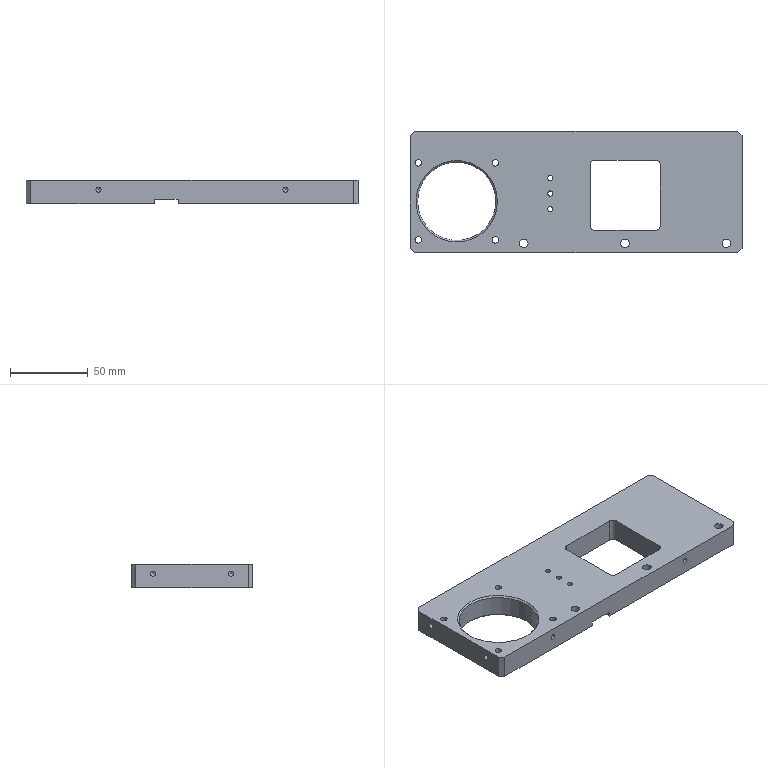Part | 1 solid | 57 faces | box 213 x 78 x 15 mm | volume 181371 mm3 | cylinder 26 | plane 21 | cone 10 | commonest cylinder face diameters 3.3 x11 4.2 x4 6 x4 5.5 x3 10 x3 50.3 x1
STEP:
#1=CARTESIAN_POINT('',(-38.5,-33.,-2.1));
#2=VERTEX_POINT('',#1);
#3=CARTESIAN_POINT('',(-33.5,-33.,-2.1));
#4=DIRECTION('',(0.,0.,-1.));
#5=DIRECTION('',(-1.,0.,0.));
#6=AXIS2_PLACEMENT_3D('',#3,#4,#5);
#7=CIRCLE('',#6,5.);
#8=EDGE_CURVE('',#2,#2,#7,.T.);
#9=ORIENTED_EDGE('',*,*,#8,.T.);
#10=EDGE_LOOP('',(#9));
#11=FACE_BOUND('',#10,.T.);
#12=CARTESIAN_POINT('',(-36.25,-33.,-2.1));
#13=VERTEX_POINT('',#12);
#14=CARTESIAN_POINT('',(-33.5,-33.,-2.1));
#15=DIRECTION('',(0.,0.,-1.));
#16=DIRECTION('',(-1.,0.,0.));
#17=AXIS2_PLACEMENT_3D('',#14,#15,#16);
#18=CIRCLE('',#17,2.75);
#19=EDGE_CURVE('',#13,#13,#18,.T.);
#20=ORIENTED_EDGE('',*,*,#19,.F.);
#21=EDGE_LOOP('',(#20));
#22=FACE_BOUND('',#21,.T.);
#23=CARTESIAN_POINT('',(-30.75,-33.,-2.1));
#24=DIRECTION('',(0.,0.,1.));
#25=DIRECTION('',(1.,0.,0.));
#26=AXIS2_PLACEMENT_3D('',#23,#24,#25);
#27=PLANE('',#26);
#28=ADVANCED_FACE('',(#11,#22),#27,.F.);
#29=CARTESIAN_POINT('',(101.5,-33.,-2.1));
#30=VERTEX_POINT('',#29);
#31=CARTESIAN_POINT('',(96.5,-33.,-2.1));
#32=DIRECTION('',(0.,0.,-1.));
#33=DIRECTION('',(1.,0.,0.));
#34=AXIS2_PLACEMENT_3D('',#31,#32,#33);
#35=CIRCLE('',#34,5.);
#36=EDGE_CURVE('',#30,#30,#35,.T.);
#37=ORIENTED_EDGE('',*,*,#36,.T.);
#38=EDGE_LOOP('',(#37));
#39=FACE_BOUND('',#38,.T.);
#40=CARTESIAN_POINT('',(99.25,-33.,-2.1));
#41=VERTEX_POINT('',#40);
#42=CARTESIAN_POINT('',(96.5,-33.,-2.1));
#43=DIRECTION('',(0.,0.,-1.));
#44=DIRECTION('',(1.,0.,0.));
#45=AXIS2_PLACEMENT_3D('',#42,#43,#44);
#46=CIRCLE('',#45,2.75);
#47=EDGE_CURVE('',#41,#41,#46,.T.);
#48=ORIENTED_EDGE('',*,*,#47,.F.);
#49=EDGE_LOOP('',(#48));
#50=FACE_BOUND('',#49,.T.);
#51=CARTESIAN_POINT('',(-30.75,-33.,-2.1));
#52=DIRECTION('',(0.,0.,1.));
#53=DIRECTION('',(1.,0.,0.));
#54=AXIS2_PLACEMENT_3D('',#51,#52,#53);
#55=PLANE('',#54);
#56=ADVANCED_FACE('',(#39,#50),#55,.F.);
#57=CARTESIAN_POINT('',(36.5,-33.,-2.1));
#58=VERTEX_POINT('',#57);
#59=CARTESIAN_POINT('',(31.5,-33.,-2.1));
#60=DIRECTION('',(0.,0.,-1.));
#61=DIRECTION('',(1.,0.,0.));
#62=AXIS2_PLACEMENT_3D('',#59,#60,#61);
#63=CIRCLE('',#62,5.);
#64=EDGE_CURVE('',#58,#58,#63,.T.);
#65=ORIENTED_EDGE('',*,*,#64,.T.);
#66=EDGE_LOOP('',(#65));
#67=FACE_BOUND('',#66,.T.);
#68=CARTESIAN_POINT('',(34.25,-33.,-2.1));
#69=VERTEX_POINT('',#68);
#70=CARTESIAN_POINT('',(31.5,-33.,-2.1));
#71=DIRECTION('',(0.,0.,-1.));
#72=DIRECTION('',(1.,0.,0.));
#73=AXIS2_PLACEMENT_3D('',#70,#71,#72);
#74=CIRCLE('',#73,2.75);
#75=EDGE_CURVE('',#69,#69,#74,.T.);
#76=ORIENTED_EDGE('',*,*,#75,.F.);
#77=EDGE_LOOP('',(#76));
#78=FACE_BOUND('',#77,.T.);
#79=CARTESIAN_POINT('',(-30.75,-33.,-2.1));
#80=DIRECTION('',(0.,0.,1.));
#81=DIRECTION('',(1.,0.,0.));
#82=AXIS2_PLACEMENT_3D('',#79,#80,#81);
#83=PLANE('',#82);
#84=ADVANCED_FACE('',(#67,#78),#83,.F.);
#85=CARTESIAN_POINT('',(106.5,36.,7.5));
#86=VERTEX_POINT('',#85);
#87=CARTESIAN_POINT('',(103.5,39.,7.5));
#88=VERTEX_POINT('',#87);
#89=CARTESIAN_POINT('',(71.25,71.25,7.5));
#90=DIRECTION('',(-0.7071,0.7071,0.));
#91=VECTOR('',#90,1000.);
#92=LINE('',#89,#91);
#93=EDGE_CURVE('',#86,#88,#92,.T.);
#94=ORIENTED_EDGE('',*,*,#93,.F.);
#95=CARTESIAN_POINT('',(106.5,36.,-7.5));
#96=VERTEX_POINT('',#95);
#97=CARTESIAN_POINT('',(106.5,36.,7.5));
#98=DIRECTION('',(0.,0.,1.));
#99=VECTOR('',#98,1000.);
#100=LINE('',#97,#99);
#101=EDGE_CURVE('',#96,#86,#100,.T.);
#102=ORIENTED_EDGE('',*,*,#101,.F.);
#103=CARTESIAN_POINT('',(103.5,39.,-7.5));
#104=VERTEX_POINT('',#103);
#105=CARTESIAN_POINT('',(103.5,39.,-7.5));
#106=DIRECTION('',(0.7071,-0.7071,0.));
#107=VECTOR('',#106,1000.);
#108=LINE('',#105,#107);
#109=EDGE_CURVE('',#104,#96,#108,.T.);
#110=ORIENTED_EDGE('',*,*,#109,.F.);
#111=CARTESIAN_POINT('',(103.5,39.,7.5));
#112=DIRECTION('',(0.,0.,-1.));
#113=VECTOR('',#112,1000.);
#114=LINE('',#111,#113);
#115=EDGE_CURVE('',#88,#104,#114,.T.);
#116=ORIENTED_EDGE('',*,*,#115,.F.);
#117=EDGE_LOOP('',(#94,#102,#110,#116));
#118=FACE_BOUND('',#117,.T.);
#119=CARTESIAN_POINT('',(103.5,39.,7.5));
#120=DIRECTION('',(-0.7071,-0.7071,0.));
#121=DIRECTION('',(0.,0.,-1.));
#122=AXIS2_PLACEMENT_3D('',#119,#120,#121);
#123=PLANE('',#122);
#124=ADVANCED_FACE('',(#118),#123,.F.);
#125=CARTESIAN_POINT('',(103.5,-39.,7.5));
#126=VERTEX_POINT('',#125);
#127=CARTESIAN_POINT('',(106.5,-36.,7.5));
#128=VERTEX_POINT('',#127);
#129=CARTESIAN_POINT('',(71.25,-71.25,7.5));
#130=DIRECTION('',(0.7071,0.7071,0.));
#131=VECTOR('',#130,1000.);
#132=LINE('',#129,#131);
#133=EDGE_CURVE('',#126,#128,#132,.T.);
#134=ORIENTED_EDGE('',*,*,#133,.F.);
#135=CARTESIAN_POINT('',(103.5,-39.,-7.5));
#136=VERTEX_POINT('',#135);
#137=CARTESIAN_POINT('',(103.5,-39.,7.5));
#138=DIRECTION('',(0.,0.,1.));
#139=VECTOR('',#138,1000.);
#140=LINE('',#137,#139);
#141=EDGE_CURVE('',#136,#126,#140,.T.);
#142=ORIENTED_EDGE('',*,*,#141,.F.);
#143=CARTESIAN_POINT('',(106.5,-36.,-7.5));
#144=VERTEX_POINT('',#143);
#145=CARTESIAN_POINT('',(106.5,-36.,-7.5));
#146=DIRECTION('',(-0.7071,-0.7071,0.));
#147=VECTOR('',#146,1000.);
#148=LINE('',#145,#147);
#149=EDGE_CURVE('',#144,#136,#148,.T.);
#150=ORIENTED_EDGE('',*,*,#149,.F.);
#151=CARTESIAN_POINT('',(106.5,-36.,7.5));
#152=DIRECTION('',(0.,0.,-1.));
#153=VECTOR('',#152,1000.);
#154=LINE('',#151,#153);
#155=EDGE_CURVE('',#128,#144,#154,.T.);
#156=ORIENTED_EDGE('',*,*,#155,.F.);
#157=EDGE_LOOP('',(#134,#142,#150,#156));
#158=FACE_BOUND('',#157,.T.);
#159=CARTESIAN_POINT('',(106.5,-36.,7.5));
#160=DIRECTION('',(-0.7071,0.7071,0.));
#161=DIRECTION('',(0.,0.,-1.));
#162=AXIS2_PLACEMENT_3D('',#159,#160,#161);
#163=PLANE('',#162);
#164=ADVANCED_FACE('',(#158),#163,.F.);
#165=CARTESIAN_POINT('',(-103.5,39.,7.5));
#166=VERTEX_POINT('',#165);
#167=CARTESIAN_POINT('',(-106.5,36.,7.5));
#168=VERTEX_POINT('',#167);
#169=CARTESIAN_POINT('',(-71.25,71.25,7.5));
#170=DIRECTION('',(-0.7071,-0.7071,0.));
#171=VECTOR('',#170,1000.);
#172=LINE('',#169,#171);
#173=EDGE_CURVE('',#166,#168,#172,.T.);
#174=ORIENTED_EDGE('',*,*,#173,.F.);
#175=CARTESIAN_POINT('',(-103.5,39.,-7.5));
#176=VERTEX_POINT('',#175);
#177=CARTESIAN_POINT('',(-103.5,39.,7.5));
#178=DIRECTION('',(0.,0.,1.));
#179=VECTOR('',#178,1000.);
#180=LINE('',#177,#179);
#181=EDGE_CURVE('',#176,#166,#180,.T.);
#182=ORIENTED_EDGE('',*,*,#181,.F.);
#183=CARTESIAN_POINT('',(-106.5,36.,-7.5));
#184=VERTEX_POINT('',#183);
#185=CARTESIAN_POINT('',(-106.5,36.,-7.5));
#186=DIRECTION('',(0.7071,0.7071,0.));
#187=VECTOR('',#186,1000.);
#188=LINE('',#185,#187);
#189=EDGE_CURVE('',#184,#176,#188,.T.);
#190=ORIENTED_EDGE('',*,*,#189,.F.);
#191=CARTESIAN_POINT('',(-106.5,36.,7.5));
#192=DIRECTION('',(0.,0.,-1.));
#193=VECTOR('',#192,1000.);
#194=LINE('',#191,#193);
#195=EDGE_CURVE('',#168,#184,#194,.T.);
#196=ORIENTED_EDGE('',*,*,#195,.F.);
#197=EDGE_LOOP('',(#174,#182,#190,#196));
#198=FACE_BOUND('',#197,.T.);
#199=CARTESIAN_POINT('',(-106.5,36.,7.5));
#200=DIRECTION('',(0.7071,-0.7071,0.));
#201=DIRECTION('',(0.,0.,-1.));
#202=AXIS2_PLACEMENT_3D('',#199,#200,#201);
#203=PLANE('',#202);
#204=ADVANCED_FACE('',(#198),#203,.F.);
#205=CARTESIAN_POINT('',(-106.5,-36.,7.5));
#206=VERTEX_POINT('',#205);
#207=CARTESIAN_POINT('',(-103.5,-39.,7.5));
#208=VERTEX_POINT('',#207);
#209=CARTESIAN_POINT('',(-71.25,-71.25,7.5));
#210=DIRECTION('',(0.7071,-0.7071,0.));
#211=VECTOR('',#210,1000.);
#212=LINE('',#209,#211);
#213=EDGE_CURVE('',#206,#208,#212,.T.);
#214=ORIENTED_EDGE('',*,*,#213,.F.);
#215=CARTESIAN_POINT('',(-106.5,-36.,-7.5));
#216=VERTEX_POINT('',#215);
#217=CARTESIAN_POINT('',(-106.5,-36.,7.5));
#218=DIRECTION('',(0.,0.,1.));
#219=VECTOR('',#218,1000.);
#220=LINE('',#217,#219);
#221=EDGE_CURVE('',#216,#206,#220,.T.);
#222=ORIENTED_EDGE('',*,*,#221,.F.);
#223=CARTESIAN_POINT('',(-103.5,-39.,-7.5));
#224=VERTEX_POINT('',#223);
#225=CARTESIAN_POINT('',(-103.5,-39.,-7.5));
#226=DIRECTION('',(-0.7071,0.7071,0.));
#227=VECTOR('',#226,1000.);
#228=LINE('',#225,#227);
#229=EDGE_CURVE('',#224,#216,#228,.T.);
#230=ORIENTED_EDGE('',*,*,#229,.F.);
#231=CARTESIAN_POINT('',(-103.5,-39.,7.5));
#232=DIRECTION('',(0.,0.,-1.));
#233=VECTOR('',#232,1000.);
#234=LINE('',#231,#233);
#235=EDGE_CURVE('',#208,#224,#234,.T.);
#236=ORIENTED_EDGE('',*,*,#235,.F.);
#237=EDGE_LOOP('',(#214,#222,#230,#236));
#238=FACE_BOUND('',#237,.T.);
#239=CARTESIAN_POINT('',(-103.5,-39.,7.5));
#240=DIRECTION('',(0.7071,0.7071,0.));
#241=DIRECTION('',(0.,0.,-1.));
#242=AXIS2_PLACEMENT_3D('',#239,#240,#241);
#243=PLANE('',#242);
#244=ADVANCED_FACE('',(#238),#243,.F.);
#245=CARTESIAN_POINT('',(51.,20.5,7.5));
#246=VERTEX_POINT('',#245);
#247=CARTESIAN_POINT('',(54.,17.5,7.5));
#248=VERTEX_POINT('',#247);
#249=CARTESIAN_POINT('',(51.,17.5,7.5));
#250=DIRECTION('',(0.,0.,-1.));
#251=DIRECTION('',(1.,0.,0.));
#252=AXIS2_PLACEMENT_3D('',#249,#250,#251);
#253=CIRCLE('',#252,3.);
#254=EDGE_CURVE('',#246,#248,#253,.T.);
#255=ORIENTED_EDGE('',*,*,#254,.F.);
#256=CARTESIAN_POINT('',(51.,20.5,-7.5));
#257=VERTEX_POINT('',#256);
#258=CARTESIAN_POINT('',(51.,20.5,7.5));
#259=DIRECTION('',(0.,0.,1.));
#260=VECTOR('',#259,1000.);
#261=LINE('',#258,#260);
#262=EDGE_CURVE('',#257,#246,#261,.T.);
#263=ORIENTED_EDGE('',*,*,#262,.F.);
#264=CARTESIAN_POINT('',(54.,17.5,-7.5));
#265=VERTEX_POINT('',#264);
#266=CARTESIAN_POINT('',(51.,17.5,-7.5));
#267=DIRECTION('',(0.,0.,1.));
#268=DIRECTION('',(1.,0.,0.));
#269=AXIS2_PLACEMENT_3D('',#266,#267,#268);
#270=CIRCLE('',#269,3.);
#271=EDGE_CURVE('',#265,#257,#270,.T.);
#272=ORIENTED_EDGE('',*,*,#271,.F.);
#273=CARTESIAN_POINT('',(54.,17.5,-7.5));
#274=DIRECTION('',(0.,0.,-1.));
#275=VECTOR('',#274,1000.);
#276=LINE('',#273,#275);
#277=EDGE_CURVE('',#248,#265,#276,.T.);
#278=ORIENTED_EDGE('',*,*,#277,.F.);
#279=EDGE_LOOP('',(#255,#263,#272,#278));
#280=FACE_BOUND('',#279,.T.);
#281=CARTESIAN_POINT('',(51.,17.5,7.5));
#282=DIRECTION('',(0.,0.,1.));
#283=DIRECTION('',(1.,0.,0.));
#284=AXIS2_PLACEMENT_3D('',#281,#282,#283);
#285=CYLINDRICAL_SURFACE('',#284,3.);
#286=ADVANCED_FACE('',(#280),#285,.F.);
#287=CARTESIAN_POINT('',(54.,-21.5,7.5));
#288=VERTEX_POINT('',#287);
#289=CARTESIAN_POINT('',(51.,-24.5,7.5));
#290=VERTEX_POINT('',#289);
#291=CARTESIAN_POINT('',(51.,-21.5,7.5));
#292=DIRECTION('',(0.,0.,-1.));
#293=DIRECTION('',(1.,0.,0.));
#294=AXIS2_PLACEMENT_3D('',#291,#292,#293);
#295=CIRCLE('',#294,3.);
#296=EDGE_CURVE('',#288,#290,#295,.T.);
#297=ORIENTED_EDGE('',*,*,#296,.F.);
#298=CARTESIAN_POINT('',(54.,-21.5,-7.5));
#299=VERTEX_POINT('',#298);
#300=CARTESIAN_POINT('',(54.,-21.5,7.5));
#301=DIRECTION('',(0.,0.,1.));
#302=VECTOR('',#301,1000.);
#303=LINE('',#300,#302);
#304=EDGE_CURVE('',#299,#288,#303,.T.);
#305=ORIENTED_EDGE('',*,*,#304,.F.);
#306=CARTESIAN_POINT('',(51.,-24.5,-7.5));
#307=VERTEX_POINT('',#306);
#308=CARTESIAN_POINT('',(51.,-21.5,-7.5));
#309=DIRECTION('',(0.,0.,1.));
#310=DIRECTION('',(1.,0.,0.));
#311=AXIS2_PLACEMENT_3D('',#308,#309,#310);
#312=CIRCLE('',#311,3.);
#313=EDGE_CURVE('',#307,#299,#312,.T.);
#314=ORIENTED_EDGE('',*,*,#313,.F.);
#315=CARTESIAN_POINT('',(51.,-24.5,-7.5));
#316=DIRECTION('',(0.,0.,-1.));
#317=VECTOR('',#316,1000.);
#318=LINE('',#315,#317);
#319=EDGE_CURVE('',#290,#307,#318,.T.);
#320=ORIENTED_EDGE('',*,*,#319,.F.);
#321=EDGE_LOOP('',(#297,#305,#314,#320));
#322=FACE_BOUND('',#321,.T.);
#323=CARTESIAN_POINT('',(51.,-21.5,7.5));
#324=DIRECTION('',(0.,0.,1.));
#325=DIRECTION('',(1.,0.,0.));
#326=AXIS2_PLACEMENT_3D('',#323,#324,#325);
#327=CYLINDRICAL_SURFACE('',#326,3.);
#328=ADVANCED_FACE('',(#322),#327,.F.);
#329=CARTESIAN_POINT('',(12.,-24.5,7.5));
#330=VERTEX_POINT('',#329);
#331=CARTESIAN_POINT('',(9.,-21.5,7.5));
#332=VERTEX_POINT('',#331);
#333=CARTESIAN_POINT('',(12.,-21.5,7.5));
#334=DIRECTION('',(0.,0.,-1.));
#335=DIRECTION('',(1.,0.,0.));
#336=AXIS2_PLACEMENT_3D('',#333,#334,#335);
#337=CIRCLE('',#336,3.);
#338=EDGE_CURVE('',#330,#332,#337,.T.);
#339=ORIENTED_EDGE('',*,*,#338,.F.);
#340=CARTESIAN_POINT('',(12.,-24.5,-7.5));
#341=VERTEX_POINT('',#340);
#342=CARTESIAN_POINT('',(12.,-24.5,7.5));
#343=DIRECTION('',(0.,0.,1.));
#344=VECTOR('',#343,1000.);
#345=LINE('',#342,#344);
#346=EDGE_CURVE('',#341,#330,#345,.T.);
#347=ORIENTED_EDGE('',*,*,#346,.F.);
#348=CARTESIAN_POINT('',(9.,-21.5,-7.5));
#349=VERTEX_POINT('',#348);
#350=CARTESIAN_POINT('',(12.,-21.5,-7.5));
#351=DIRECTION('',(0.,0.,1.));
#352=DIRECTION('',(1.,0.,0.));
#353=AXIS2_PLACEMENT_3D('',#350,#351,#352);
#354=CIRCLE('',#353,3.);
#355=EDGE_CURVE('',#349,#341,#354,.T.);
#356=ORIENTED_EDGE('',*,*,#355,.F.);
#357=CARTESIAN_POINT('',(9.,-21.5,-7.5));
#358=DIRECTION('',(0.,0.,-1.));
#359=VECTOR('',#358,1000.);
#360=LINE('',#357,#359);
#361=EDGE_CURVE('',#332,#349,#360,.T.);
#362=ORIENTED_EDGE('',*,*,#361,.F.);
#363=EDGE_LOOP('',(#339,#347,#356,#362));
#364=FACE_BOUND('',#363,.T.);
#365=CARTESIAN_POINT('',(12.,-21.5,7.5));
#366=DIRECTION('',(0.,0.,1.));
#367=DIRECTION('',(1.,0.,0.));
#368=AXIS2_PLACEMENT_3D('',#365,#366,#367);
#369=CYLINDRICAL_SURFACE('',#368,3.);
#370=ADVANCED_FACE('',(#364),#369,.F.);
#371=CARTESIAN_POINT('',(9.,17.5,7.5));
#372=VERTEX_POINT('',#371);
#373=CARTESIAN_POINT('',(12.,20.5,7.5));
#374=VERTEX_POINT('',#373);
#375=CARTESIAN_POINT('',(12.,17.5,7.5));
#376=DIRECTION('',(0.,0.,-1.));
#377=DIRECTION('',(1.,0.,0.));
#378=AXIS2_PLACEMENT_3D('',#375,#376,#377);
#379=CIRCLE('',#378,3.);
#380=EDGE_CURVE('',#372,#374,#379,.T.);
#381=ORIENTED_EDGE('',*,*,#380,.F.);
#382=CARTESIAN_POINT('',(9.,17.5,-7.5));
#383=VERTEX_POINT('',#382);
#384=CARTESIAN_POINT('',(9.,17.5,7.5));
#385=DIRECTION('',(0.,0.,1.));
#386=VECTOR('',#385,1000.);
#387=LINE('',#384,#386);
#388=EDGE_CURVE('',#383,#372,#387,.T.);
#389=ORIENTED_EDGE('',*,*,#388,.F.);
#390=CARTESIAN_POINT('',(12.,20.5,-7.5));
#391=VERTEX_POINT('',#390);
#392=CARTESIAN_POINT('',(12.,17.5,-7.5));
#393=DIRECTION('',(0.,0.,1.));
#394=DIRECTION('',(1.,0.,0.));
#395=AXIS2_PLACEMENT_3D('',#392,#393,#394);
#396=CIRCLE('',#395,3.);
#397=EDGE_CURVE('',#391,#383,#396,.T.);
#398=ORIENTED_EDGE('',*,*,#397,.F.);
#399=CARTESIAN_POINT('',(12.,20.5,-7.5));
#400=DIRECTION('',(0.,0.,-1.));
#401=VECTOR('',#400,1000.);
#402=LINE('',#399,#401);
#403=EDGE_CURVE('',#374,#391,#402,.T.);
#404=ORIENTED_EDGE('',*,*,#403,.F.);
#405=EDGE_LOOP('',(#381,#389,#398,#404));
#406=FACE_BOUND('',#405,.T.);
#407=CARTESIAN_POINT('',(12.,17.5,7.5));
#408=DIRECTION('',(0.,0.,1.));
#409=DIRECTION('',(1.,0.,0.));
#410=AXIS2_PLACEMENT_3D('',#407,#408,#409);
#411=CYLINDRICAL_SURFACE('',#410,3.);
#412=ADVANCED_FACE('',(#406),#411,.F.);
#413=CARTESIAN_POINT('',(54.,20.5,7.5));
#414=DIRECTION('',(1.,0.,0.));
#415=VECTOR('',#414,1000.);
#416=LINE('',#413,#415);
#417=EDGE_CURVE('',#374,#246,#416,.T.);
#418=ORIENTED_EDGE('',*,*,#417,.F.);
#419=ORIENTED_EDGE('',*,*,#403,.T.);
#420=CARTESIAN_POINT('',(54.,20.5,-7.5));
#421=DIRECTION('',(1.,0.,0.));
#422=VECTOR('',#421,1000.);
#423=LINE('',#420,#422);
#424=EDGE_CURVE('',#391,#257,#423,.T.);
#425=ORIENTED_EDGE('',*,*,#424,.T.);
#426=ORIENTED_EDGE('',*,*,#262,.T.);
#427=EDGE_LOOP('',(#418,#419,#425,#426));
#428=FACE_BOUND('',#427,.T.);
#429=CARTESIAN_POINT('',(54.,20.5,7.5));
#430=DIRECTION('',(0.,1.,0.));
#431=DIRECTION('',(0.,0.,1.));
#432=AXIS2_PLACEMENT_3D('',#429,#430,#431);
#433=PLANE('',#432);
#434=ADVANCED_FACE('',(#428),#433,.F.);
#435=CARTESIAN_POINT('',(54.,20.5,-7.5));
#436=DIRECTION('',(0.,-1.,0.));
#437=VECTOR('',#436,1000.);
#438=LINE('',#435,#437);
#439=EDGE_CURVE('',#265,#299,#438,.T.);
#440=ORIENTED_EDGE('',*,*,#439,.T.);
#441=ORIENTED_EDGE('',*,*,#304,.T.);
#442=CARTESIAN_POINT('',(54.,20.5,7.5));
#443=DIRECTION('',(0.,-1.,0.));
#444=VECTOR('',#443,1000.);
#445=LINE('',#442,#444);
#446=EDGE_CURVE('',#248,#288,#445,.T.);
#447=ORIENTED_EDGE('',*,*,#446,.F.);
#448=ORIENTED_EDGE('',*,*,#277,.T.);
#449=EDGE_LOOP('',(#440,#441,#447,#448));
#450=FACE_BOUND('',#449,.T.);
#451=CARTESIAN_POINT('',(54.,20.5,7.5));
#452=DIRECTION('',(1.,0.,0.));
#453=DIRECTION('',(0.,1.,0.));
#454=AXIS2_PLACEMENT_3D('',#451,#452,#453);
#455=PLANE('',#454);
#456=ADVANCED_FACE('',(#450),#455,.F.);
#457=CARTESIAN_POINT('',(54.,-24.5,-7.5));
#458=DIRECTION('',(-1.,0.,0.));
#459=VECTOR('',#458,1000.);
#460=LINE('',#457,#459);
#461=EDGE_CURVE('',#307,#341,#460,.T.);
#462=ORIENTED_EDGE('',*,*,#461,.T.);
#463=ORIENTED_EDGE('',*,*,#346,.T.);
#464=CARTESIAN_POINT('',(54.,-24.5,7.5));
#465=DIRECTION('',(-1.,0.,0.));
#466=VECTOR('',#465,1000.);
#467=LINE('',#464,#466);
#468=EDGE_CURVE('',#290,#330,#467,.T.);
#469=ORIENTED_EDGE('',*,*,#468,.F.);
#470=ORIENTED_EDGE('',*,*,#319,.T.);
#471=EDGE_LOOP('',(#462,#463,#469,#470));
#472=FACE_BOUND('',#471,.T.);
#473=CARTESIAN_POINT('',(54.,-24.5,7.5));
#474=DIRECTION('',(0.,-1.,0.));
#475=DIRECTION('',(0.,0.,-1.));
#476=AXIS2_PLACEMENT_3D('',#473,#474,#475);
#477=PLANE('',#476);
#478=ADVANCED_FACE('',(#472),#477,.F.);
#479=CARTESIAN_POINT('',(9.,20.5,-7.5));
#480=DIRECTION('',(0.,1.,0.));
#481=VECTOR('',#480,1000.);
#482=LINE('',#479,#481);
#483=EDGE_CURVE('',#349,#383,#482,.T.);
#484=ORIENTED_EDGE('',*,*,#483,.T.);
#485=ORIENTED_EDGE('',*,*,#388,.T.);
#486=CARTESIAN_POINT('',(9.,20.5,7.5));
#487=DIRECTION('',(0.,1.,0.));
#488=VECTOR('',#487,1000.);
#489=LINE('',#486,#488);
#490=EDGE_CURVE('',#332,#372,#489,.T.);
#491=ORIENTED_EDGE('',*,*,#490,.F.);
#492=ORIENTED_EDGE('',*,*,#361,.T.);
#493=EDGE_LOOP('',(#484,#485,#491,#492));
#494=FACE_BOUND('',#493,.T.);
#495=CARTESIAN_POINT('',(9.,20.5,7.5));
#496=DIRECTION('',(-1.,0.,0.));
#497=DIRECTION('',(0.,-1.,0.));
#498=AXIS2_PLACEMENT_3D('',#495,#496,#497);
#499=PLANE('',#498);
#500=ADVANCED_FACE('',(#494),#499,.F.);
#501=CARTESIAN_POINT('',(-8.95,39.,-4.5));
#502=VERTEX_POINT('',#501);
#503=CARTESIAN_POINT('',(-8.95,-39.,-4.5));
#504=VERTEX_POINT('',#503);
#505=CARTESIAN_POINT('',(-8.95,39.,-4.5));
#506=DIRECTION('',(0.,-1.,0.));
#507=VECTOR('',#506,1000.);
#508=LINE('',#505,#507);
#509=EDGE_CURVE('',#502,#504,#508,.T.);
#510=ORIENTED_EDGE('',*,*,#509,.T.);
#511=CARTESIAN_POINT('',(-24.05,-39.,-4.5));
#512=VERTEX_POINT('',#511);
#513=CARTESIAN_POINT('',(-8.95,-39.,-4.5));
#514=DIRECTION('',(-1.,0.,0.));
#515=VECTOR('',#514,1000.);
#516=LINE('',#513,#515);
#517=EDGE_CURVE('',#504,#512,#516,.T.);
#518=ORIENTED_EDGE('',*,*,#517,.T.);
#519=CARTESIAN_POINT('',(-24.05,39.,-4.5));
#520=VERTEX_POINT('',#519);
#521=CARTESIAN_POINT('',(-24.05,39.,-4.5));
#522=DIRECTION('',(0.,1.,0.));
#523=VECTOR('',#522,1000.);
#524=LINE('',#521,#523);
#525=EDGE_CURVE('',#512,#520,#524,.T.);
#526=ORIENTED_EDGE('',*,*,#525,.T.);
#527=CARTESIAN_POINT('',(-8.95,39.,-4.5));
#528=DIRECTION('',(1.,0.,0.));
#529=VECTOR('',#528,1000.);
#530=LINE('',#527,#529);
#531=EDGE_CURVE('',#520,#502,#530,.T.);
#532=ORIENTED_EDGE('',*,*,#531,.T.);
#533=EDGE_LOOP('',(#510,#518,#526,#532));
#534=FACE_BOUND('',#533,.T.);
#535=CARTESIAN_POINT('',(-18.15,-11.,-4.5));
#536=VERTEX_POINT('',#535);
#537=CARTESIAN_POINT('',(-16.5,-11.,-4.5));
#538=DIRECTION('',(0.,0.,-1.));
#539=DIRECTION('',(-1.,0.,0.));
#540=AXIS2_PLACEMENT_3D('',#537,#538,#539);
#541=CIRCLE('',#540,1.65);
#542=EDGE_CURVE('',#536,#536,#541,.T.);
#543=ORIENTED_EDGE('',*,*,#542,.F.);
#544=EDGE_LOOP('',(#543));
#545=FACE_BOUND('',#544,.T.);
#546=CARTESIAN_POINT('',(-18.15,9.,-4.5));
#547=VERTEX_POINT('',#546);
#548=CARTESIAN_POINT('',(-16.5,9.,-4.5));
#549=DIRECTION('',(0.,0.,-1.));
#550=DIRECTION('',(-1.,0.,0.));
#551=AXIS2_PLACEMENT_3D('',#548,#549,#550);
#552=CIRCLE('',#551,1.65);
#553=EDGE_CURVE('',#547,#547,#552,.T.);
#554=ORIENTED_EDGE('',*,*,#553,.F.);
#555=EDGE_LOOP('',(#554));
#556=FACE_BOUND('',#555,.T.);
#557=CARTESIAN_POINT('',(-18.15,-1.,-4.5));
#558=VERTEX_POINT('',#557);
#559=CARTESIAN_POINT('',(-16.5,-1.,-4.5));
#560=DIRECTION('',(0.,0.,-1.));
#561=DIRECTION('',(-1.,0.,0.));
#562=AXIS2_PLACEMENT_3D('',#559,#560,#561);
#563=CIRCLE('',#562,1.65);
#564=EDGE_CURVE('',#558,#558,#563,.T.);
#565=ORIENTED_EDGE('',*,*,#564,.F.);
#566=EDGE_LOOP('',(#565));
#567=FACE_BOUND('',#566,.T.);
#568=CARTESIAN_POINT('',(0.,0.,-4.5));
#569=DIRECTION('',(0.,0.,-1.));
#570=DIRECTION('',(-1.,0.,0.));
#571=AXIS2_PLACEMENT_3D('',#568,#569,#570);
#572=PLANE('',#571);
#573=ADVANCED_FACE('',(#534,#545,#556,#567),#572,.T.);
#574=CARTESIAN_POINT('',(-24.05,-39.,-7.5));
#575=VERTEX_POINT('',#574);
#576=CARTESIAN_POINT('',(-24.05,39.,-7.5));
#577=VERTEX_POINT('',#576);
#578=CARTESIAN_POINT('',(-24.05,39.,-7.5));
#579=DIRECTION('',(0.,1.,0.));
#580=VECTOR('',#579,1000.);
#581=LINE('',#578,#580);
#582=EDGE_CURVE('',#575,#577,#581,.T.);
#583=ORIENTED_EDGE('',*,*,#582,.T.);
#584=CARTESIAN_POINT('',(-24.05,39.,-4.5));
#585=DIRECTION('',(0.,0.,-1.));
#586=VECTOR('',#585,1000.);
#587=LINE('',#584,#586);
#588=EDGE_CURVE('',#520,#577,#587,.T.);
#589=ORIENTED_EDGE('',*,*,#588,.F.);
#590=ORIENTED_EDGE('',*,*,#525,.F.);
#591=CARTESIAN_POINT('',(-24.05,-39.,-4.5));
#592=DIRECTION('',(0.,0.,-1.));
#593=VECTOR('',#592,1000.);
#594=LINE('',#591,#593);
#595=EDGE_CURVE('',#512,#575,#594,.T.);
#596=ORIENTED_EDGE('',*,*,#595,.T.);
#597=EDGE_LOOP('',(#583,#589,#590,#596));
#598=FACE_BOUND('',#597,.T.);
#599=CARTESIAN_POINT('',(-24.05,39.,-4.5));
#600=DIRECTION('',(-1.,0.,0.));
#601=DIRECTION('',(0.,-1.,0.));
#602=AXIS2_PLACEMENT_3D('',#599,#600,#601);
#603=PLANE('',#602);
#604=ADVANCED_FACE('',(#598),#603,.F.);
#605=CARTESIAN_POINT('',(-8.95,39.,-7.5));
#606=VERTEX_POINT('',#605);
#607=CARTESIAN_POINT('',(-8.95,-39.,-7.5));
#608=VERTEX_POINT('',#607);
#609=CARTESIAN_POINT('',(-8.95,39.,-7.5));
#610=DIRECTION('',(0.,-1.,0.));
#611=VECTOR('',#610,1000.);
#612=LINE('',#609,#611);
#613=EDGE_CURVE('',#606,#608,#612,.T.);
#614=ORIENTED_EDGE('',*,*,#613,.T.);
#615=CARTESIAN_POINT('',(-8.95,-39.,-4.5));
#616=DIRECTION('',(0.,0.,-1.));
#617=VECTOR('',#616,1000.);
#618=LINE('',#615,#617);
#619=EDGE_CURVE('',#504,#608,#618,.T.);
#620=ORIENTED_EDGE('',*,*,#619,.F.);
#621=ORIENTED_EDGE('',*,*,#509,.F.);
#622=CARTESIAN_POINT('',(-8.95,39.,-4.5));
#623=DIRECTION('',(0.,0.,-1.));
#624=VECTOR('',#623,1000.);
#625=LINE('',#622,#624);
#626=EDGE_CURVE('',#502,#606,#625,.T.);
#627=ORIENTED_EDGE('',*,*,#626,.T.);
#628=EDGE_LOOP('',(#614,#620,#621,#627));
#629=FACE_BOUND('',#628,.T.);
#630=CARTESIAN_POINT('',(-8.95,39.,-4.5));
#631=DIRECTION('',(1.,0.,0.));
#632=DIRECTION('',(0.,1.,0.));
#633=AXIS2_PLACEMENT_3D('',#630,#631,#632);
#634=PLANE('',#633);
#635=ADVANCED_FACE('',(#629),#634,.F.);
#636=CARTESIAN_POINT('',(-106.5,-39.,-7.5));
#637=DIRECTION('',(1.,0.,0.));
#638=VECTOR('',#637,1000.);
#639=LINE('',#636,#638);
#640=EDGE_CURVE('',#224,#575,#639,.T.);
#641=ORIENTED_EDGE('',*,*,#640,.F.);
#642=ORIENTED_EDGE('',*,*,#229,.T.);
#643=CARTESIAN_POINT('',(-106.5,39.,-7.5));
#644=DIRECTION('',(0.,-1.,0.));
#645=VECTOR('',#644,1000.);
#646=LINE('',#643,#645);
#647=EDGE_CURVE('',#184,#216,#646,.T.);
#648=ORIENTED_EDGE('',*,*,#647,.F.);
#649=ORIENTED_EDGE('',*,*,#189,.T.);
#650=CARTESIAN_POINT('',(-106.5,39.,-7.5));
#651=DIRECTION('',(-1.,0.,0.));
#652=VECTOR('',#651,1000.);
#653=LINE('',#650,#652);
#654=EDGE_CURVE('',#577,#176,#653,.T.);
#655=ORIENTED_EDGE('',*,*,#654,.F.);
#656=ORIENTED_EDGE('',*,*,#582,.F.);
#657=EDGE_LOOP('',(#641,#642,#648,#649,#655,#656));
#658=FACE_BOUND('',#657,.T.);
#659=CARTESIAN_POINT('',(-99.149,-30.749,-7.5));
#660=VERTEX_POINT('',#659);
#661=CARTESIAN_POINT('',(-101.249,-30.749,-7.5));
#662=DIRECTION('',(0.,0.,1.));
#663=DIRECTION('',(1.,0.,0.));
#664=AXIS2_PLACEMENT_3D('',#661,#662,#663);
#665=CIRCLE('',#664,2.1);
#666=EDGE_CURVE('',#660,#660,#665,.T.);
#667=ORIENTED_EDGE('',*,*,#666,.T.);
#668=EDGE_LOOP('',(#667));
#669=FACE_BOUND('',#668,.T.);
#670=CARTESIAN_POINT('',(-49.651,-30.749,-7.5));
#671=VERTEX_POINT('',#670);
#672=CARTESIAN_POINT('',(-51.751,-30.749,-7.5));
#673=DIRECTION('',(0.,0.,1.));
#674=DIRECTION('',(1.,0.,0.));
#675=AXIS2_PLACEMENT_3D('',#672,#673,#674);
#676=CIRCLE('',#675,2.1);
#677=EDGE_CURVE('',#671,#671,#676,.T.);
#678=ORIENTED_EDGE('',*,*,#677,.T.);
#679=EDGE_LOOP('',(#678));
#680=FACE_BOUND('',#679,.T.);
#681=CARTESIAN_POINT('',(-49.651,18.749,-7.5));
#682=VERTEX_POINT('',#681);
#683=CARTESIAN_POINT('',(-51.751,18.749,-7.5));
#684=DIRECTION('',(0.,0.,1.));
#685=DIRECTION('',(1.,0.,0.));
#686=AXIS2_PLACEMENT_3D('',#683,#684,#685);
#687=CIRCLE('',#686,2.1);
#688=EDGE_CURVE('',#682,#682,#687,.T.);
#689=ORIENTED_EDGE('',*,*,#688,.T.);
#690=EDGE_LOOP('',(#689));
#691=FACE_BOUND('',#690,.T.);
#692=CARTESIAN_POINT('',(-99.149,18.749,-7.5));
#693=VERTEX_POINT('',#692);
#694=CARTESIAN_POINT('',(-101.249,18.749,-7.5));
#695=DIRECTION('',(0.,0.,1.));
#696=DIRECTION('',(1.,0.,0.));
#697=AXIS2_PLACEMENT_3D('',#694,#695,#696);
#698=CIRCLE('',#697,2.1);
#699=EDGE_CURVE('',#693,#693,#698,.T.);
#700=ORIENTED_EDGE('',*,*,#699,.T.);
#701=EDGE_LOOP('',(#700));
#702=FACE_BOUND('',#701,.T.);
#703=CARTESIAN_POINT('',(-38.5,-33.,-7.5));
#704=VERTEX_POINT('',#703);
#705=CARTESIAN_POINT('',(-33.5,-33.,-7.5));
#706=DIRECTION('',(0.,0.,-1.));
#707=DIRECTION('',(-1.,0.,0.));
#708=AXIS2_PLACEMENT_3D('',#705,#706,#707);
#709=CIRCLE('',#708,5.);
#710=EDGE_CURVE('',#704,#704,#709,.T.);
#711=ORIENTED_EDGE('',*,*,#710,.F.);
#712=EDGE_LOOP('',(#711));
#713=FACE_BOUND('',#712,.T.);
#714=CARTESIAN_POINT('',(-50.35,-6.,-7.5));
#715=VERTEX_POINT('',#714);
#716=CARTESIAN_POINT('',(-76.5,-6.,-7.5));
#717=DIRECTION('',(0.,0.,1.));
#718=DIRECTION('',(1.,0.,0.));
#719=AXIS2_PLACEMENT_3D('',#716,#717,#718);
#720=CIRCLE('',#719,26.15);
#721=EDGE_CURVE('',#715,#715,#720,.T.);
#722=ORIENTED_EDGE('',*,*,#721,.T.);
#723=EDGE_LOOP('',(#722));
#724=FACE_BOUND('',#723,.T.);
#725=CARTESIAN_POINT('',(0.,0.,-7.5));
#726=DIRECTION('',(0.,0.,1.));
#727=DIRECTION('',(1.,0.,0.));
#728=AXIS2_PLACEMENT_3D('',#725,#726,#727);
#729=PLANE('',#728);
#730=ADVANCED_FACE('',(#658,#669,#680,#691,#702,#713,#724),#729,.F.);
#731=CARTESIAN_POINT('',(-106.5,39.,7.5));
#732=DIRECTION('',(0.,-1.,0.));
#733=VECTOR('',#732,1000.);
#734=LINE('',#731,#733);
#735=EDGE_CURVE('',#168,#206,#734,.T.);
#736=ORIENTED_EDGE('',*,*,#735,.T.);
#737=ORIENTED_EDGE('',*,*,#213,.T.);
#738=CARTESIAN_POINT('',(-106.5,-39.,7.5));
#739=DIRECTION('',(1.,0.,0.));
#740=VECTOR('',#739,1000.);
#741=LINE('',#738,#740);
#742=EDGE_CURVE('',#208,#126,#741,.T.);
#743=ORIENTED_EDGE('',*,*,#742,.T.);
#744=ORIENTED_EDGE('',*,*,#133,.T.);
#745=CARTESIAN_POINT('',(106.5,39.,7.5));
#746=DIRECTION('',(0.,1.,0.));
#747=VECTOR('',#746,1000.);
#748=LINE('',#745,#747);
#749=EDGE_CURVE('',#128,#86,#748,.T.);
#750=ORIENTED_EDGE('',*,*,#749,.T.);
#751=ORIENTED_EDGE('',*,*,#93,.T.);
#752=CARTESIAN_POINT('',(-106.5,39.,7.5));
#753=DIRECTION('',(-1.,0.,0.));
#754=VECTOR('',#753,1000.);
#755=LINE('',#752,#754);
#756=EDGE_CURVE('',#88,#166,#755,.T.);
#757=ORIENTED_EDGE('',*,*,#756,.T.);
#758=ORIENTED_EDGE('',*,*,#173,.T.);
#759=EDGE_LOOP('',(#736,#737,#743,#744,#750,#751,#757,#758));
#760=FACE_BOUND('',#759,.T.);
#761=ORIENTED_EDGE('',*,*,#468,.T.);
#762=ORIENTED_EDGE('',*,*,#338,.T.);
#763=ORIENTED_EDGE('',*,*,#490,.T.);
#764=ORIENTED_EDGE('',*,*,#380,.T.);
#765=ORIENTED_EDGE('',*,*,#417,.T.);
#766=ORIENTED_EDGE('',*,*,#254,.T.);
#767=ORIENTED_EDGE('',*,*,#446,.T.);
#768=ORIENTED_EDGE('',*,*,#296,.T.);
#769=EDGE_LOOP('',(#761,#762,#763,#764,#765,#766,#767,#768));
#770=FACE_BOUND('',#769,.T.);
#771=CARTESIAN_POINT('',(-99.149,-30.749,7.5));
#772=VERTEX_POINT('',#771);
#773=CARTESIAN_POINT('',(-101.249,-30.749,7.5));
#774=DIRECTION('',(0.,0.,1.));
#775=DIRECTION('',(1.,0.,0.));
#776=AXIS2_PLACEMENT_3D('',#773,#774,#775);
#777=CIRCLE('',#776,2.1);
#778=EDGE_CURVE('',#772,#772,#777,.T.);
#779=ORIENTED_EDGE('',*,*,#778,.F.);
#780=EDGE_LOOP('',(#779));
#781=FACE_BOUND('',#780,.T.);
#782=CARTESIAN_POINT('',(-49.651,-30.749,7.5));
#783=VERTEX_POINT('',#782);
#784=CARTESIAN_POINT('',(-51.751,-30.749,7.5));
#785=DIRECTION('',(0.,0.,1.));
#786=DIRECTION('',(1.,0.,0.));
#787=AXIS2_PLACEMENT_3D('',#784,#785,#786);
#788=CIRCLE('',#787,2.1);
#789=EDGE_CURVE('',#783,#783,#788,.T.);
#790=ORIENTED_EDGE('',*,*,#789,.F.);
#791=EDGE_LOOP('',(#790));
#792=FACE_BOUND('',#791,.T.);
#793=CARTESIAN_POINT('',(-49.651,18.749,7.5));
#794=VERTEX_POINT('',#793);
#795=CARTESIAN_POINT('',(-51.751,18.749,7.5));
#796=DIRECTION('',(0.,0.,1.));
#797=DIRECTION('',(1.,0.,0.));
#798=AXIS2_PLACEMENT_3D('',#795,#796,#797);
#799=CIRCLE('',#798,2.1);
#800=EDGE_CURVE('',#794,#794,#799,.T.);
#801=ORIENTED_EDGE('',*,*,#800,.F.);
#802=EDGE_LOOP('',(#801));
#803=FACE_BOUND('',#802,.T.);
#804=CARTESIAN_POINT('',(-99.149,18.749,7.5));
#805=VERTEX_POINT('',#804);
#806=CARTESIAN_POINT('',(-101.249,18.749,7.5));
#807=DIRECTION('',(0.,0.,1.));
#808=DIRECTION('',(1.,0.,0.));
#809=AXIS2_PLACEMENT_3D('',#806,#807,#808);
#810=CIRCLE('',#809,2.1);
#811=EDGE_CURVE('',#805,#805,#810,.T.);
#812=ORIENTED_EDGE('',*,*,#811,.F.);
#813=EDGE_LOOP('',(#812));
#814=FACE_BOUND('',#813,.T.);
#815=CARTESIAN_POINT('',(28.75,-33.,7.5));
#816=VERTEX_POINT('',#815);
#817=CARTESIAN_POINT('',(31.5,-33.,7.5));
#818=DIRECTION('',(0.,0.,-1.));
#819=DIRECTION('',(-1.,0.,0.));
#820=AXIS2_PLACEMENT_3D('',#817,#818,#819);
#821=CIRCLE('',#820,2.75);
#822=EDGE_CURVE('',#816,#816,#821,.T.);
#823=ORIENTED_EDGE('',*,*,#822,.T.);
#824=EDGE_LOOP('',(#823));
#825=FACE_BOUND('',#824,.T.);
#826=CARTESIAN_POINT('',(93.75,-33.,7.5));
#827=VERTEX_POINT('',#826);
#828=CARTESIAN_POINT('',(96.5,-33.,7.5));
#829=DIRECTION('',(0.,0.,-1.));
#830=DIRECTION('',(-1.,0.,0.));
#831=AXIS2_PLACEMENT_3D('',#828,#829,#830);
#832=CIRCLE('',#831,2.75);
#833=EDGE_CURVE('',#827,#827,#832,.T.);
#834=ORIENTED_EDGE('',*,*,#833,.T.);
#835=EDGE_LOOP('',(#834));
#836=FACE_BOUND('',#835,.T.);
#837=CARTESIAN_POINT('',(-36.25,-33.,7.5));
#838=VERTEX_POINT('',#837);
#839=CARTESIAN_POINT('',(-33.5,-33.,7.5));
#840=DIRECTION('',(0.,0.,-1.));
#841=DIRECTION('',(-1.,0.,0.));
#842=AXIS2_PLACEMENT_3D('',#839,#840,#841);
#843=CIRCLE('',#842,2.75);
#844=EDGE_CURVE('',#838,#838,#843,.T.);
#845=ORIENTED_EDGE('',*,*,#844,.T.);
#846=EDGE_LOOP('',(#845));
#847=FACE_BOUND('',#846,.T.);
#848=CARTESIAN_POINT('',(-18.15,-11.,7.5));
#849=VERTEX_POINT('',#848);
#850=CARTESIAN_POINT('',(-16.5,-11.,7.5));
#851=DIRECTION('',(0.,0.,-1.));
#852=DIRECTION('',(-1.,0.,0.));
#853=AXIS2_PLACEMENT_3D('',#850,#851,#852);
#854=CIRCLE('',#853,1.65);
#855=EDGE_CURVE('',#849,#849,#854,.T.);
#856=ORIENTED_EDGE('',*,*,#855,.T.);
#857=EDGE_LOOP('',(#856));
#858=FACE_BOUND('',#857,.T.);
#859=CARTESIAN_POINT('',(-18.15,9.,7.5));
#860=VERTEX_POINT('',#859);
#861=CARTESIAN_POINT('',(-16.5,9.,7.5));
#862=DIRECTION('',(0.,0.,-1.));
#863=DIRECTION('',(-1.,0.,0.));
#864=AXIS2_PLACEMENT_3D('',#861,#862,#863);
#865=CIRCLE('',#864,1.65);
#866=EDGE_CURVE('',#860,#860,#865,.T.);
#867=ORIENTED_EDGE('',*,*,#866,.T.);
#868=EDGE_LOOP('',(#867));
#869=FACE_BOUND('',#868,.T.);
#870=CARTESIAN_POINT('',(-18.15,-1.,7.5));
#871=VERTEX_POINT('',#870);
#872=CARTESIAN_POINT('',(-16.5,-1.,7.5));
#873=DIRECTION('',(0.,0.,-1.));
#874=DIRECTION('',(-1.,0.,0.));
#875=AXIS2_PLACEMENT_3D('',#872,#873,#874);
#876=CIRCLE('',#875,1.65);
#877=EDGE_CURVE('',#871,#871,#876,.T.);
#878=ORIENTED_EDGE('',*,*,#877,.T.);
#879=EDGE_LOOP('',(#878));
#880=FACE_BOUND('',#879,.T.);
#881=CARTESIAN_POINT('',(-50.35,-6.,7.5));
#882=VERTEX_POINT('',#881);
#883=CARTESIAN_POINT('',(-76.5,-6.,7.5));
#884=DIRECTION('',(0.,0.,-1.));
#885=DIRECTION('',(1.,0.,0.));
#886=AXIS2_PLACEMENT_3D('',#883,#884,#885);
#887=CIRCLE('',#886,26.15);
#888=EDGE_CURVE('',#882,#882,#887,.T.);
#889=ORIENTED_EDGE('',*,*,#888,.T.);
#890=EDGE_LOOP('',(#889));
#891=FACE_BOUND('',#890,.T.);
#892=CARTESIAN_POINT('',(0.,0.,7.5));
#893=DIRECTION('',(0.,0.,1.));
#894=DIRECTION('',(1.,0.,0.));
#895=AXIS2_PLACEMENT_3D('',#892,#893,#894);
#896=PLANE('',#895);
#897=ADVANCED_FACE('',(#760,#770,#781,#792,#803,#814,#825,#836,#847,#858,#869,#880,#891),#896,.T.);
#898=ORIENTED_EDGE('',*,*,#742,.F.);
#899=ORIENTED_EDGE('',*,*,#235,.T.);
#900=ORIENTED_EDGE('',*,*,#640,.T.);
#901=ORIENTED_EDGE('',*,*,#595,.F.);
#902=ORIENTED_EDGE('',*,*,#517,.F.);
#903=ORIENTED_EDGE('',*,*,#619,.T.);
#904=CARTESIAN_POINT('',(-106.5,-39.,-7.5));
#905=DIRECTION('',(1.,0.,0.));
#906=VECTOR('',#905,1000.);
#907=LINE('',#904,#906);
#908=EDGE_CURVE('',#608,#136,#907,.T.);
#909=ORIENTED_EDGE('',*,*,#908,.T.);
#910=ORIENTED_EDGE('',*,*,#141,.T.);
#911=EDGE_LOOP('',(#898,#899,#900,#901,#902,#903,#909,#910));
#912=FACE_BOUND('',#911,.T.);
#913=CARTESIAN_POINT('',(-60.,-39.,-0.15));
#914=VERTEX_POINT('',#913);
#915=CARTESIAN_POINT('',(-60.,-39.,1.5));
#916=DIRECTION('',(0.,-1.,0.));
#917=DIRECTION('',(0.,0.,-1.));
#918=AXIS2_PLACEMENT_3D('',#915,#916,#917);
#919=CIRCLE('',#918,1.65);
#920=EDGE_CURVE('',#914,#914,#919,.T.);
#921=ORIENTED_EDGE('',*,*,#920,.F.);
#922=EDGE_LOOP('',(#921));
#923=FACE_BOUND('',#922,.T.);
#924=CARTESIAN_POINT('',(60.,-39.,-0.15));
#925=VERTEX_POINT('',#924);
#926=CARTESIAN_POINT('',(60.,-39.,1.5));
#927=DIRECTION('',(0.,-1.,0.));
#928=DIRECTION('',(0.,0.,-1.));
#929=AXIS2_PLACEMENT_3D('',#926,#927,#928);
#930=CIRCLE('',#929,1.65);
#931=EDGE_CURVE('',#925,#925,#930,.T.);
#932=ORIENTED_EDGE('',*,*,#931,.F.);
#933=EDGE_LOOP('',(#932));
#934=FACE_BOUND('',#933,.T.);
#935=CARTESIAN_POINT('',(-106.5,-39.,7.5));
#936=DIRECTION('',(0.,1.,0.));
#937=DIRECTION('',(0.,0.,1.));
#938=AXIS2_PLACEMENT_3D('',#935,#936,#937);
#939=PLANE('',#938);
#940=ADVANCED_FACE('',(#912,#923,#934),#939,.F.);
#941=ORIENTED_EDGE('',*,*,#647,.T.);
#942=ORIENTED_EDGE('',*,*,#221,.T.);
#943=ORIENTED_EDGE('',*,*,#735,.F.);
#944=ORIENTED_EDGE('',*,*,#195,.T.);
#945=EDGE_LOOP('',(#941,#942,#943,#944));
#946=FACE_BOUND('',#945,.T.);
#947=CARTESIAN_POINT('',(-106.5,-25.,-0.15));
#948=VERTEX_POINT('',#947);
#949=CARTESIAN_POINT('',(-106.5,-25.,1.5));
#950=DIRECTION('',(-1.,0.,0.));
#951=DIRECTION('',(0.,0.,-1.));
#952=AXIS2_PLACEMENT_3D('',#949,#950,#951);
#953=CIRCLE('',#952,1.65);
#954=EDGE_CURVE('',#948,#948,#953,.T.);
#955=ORIENTED_EDGE('',*,*,#954,.F.);
#956=EDGE_LOOP('',(#955));
#957=FACE_BOUND('',#956,.T.);
#958=CARTESIAN_POINT('',(-106.5,25.,3.15));
#959=VERTEX_POINT('',#958);
#960=CARTESIAN_POINT('',(-106.5,25.,1.5));
#961=DIRECTION('',(-1.,0.,0.));
#962=DIRECTION('',(0.,0.,1.));
#963=AXIS2_PLACEMENT_3D('',#960,#961,#962);
#964=CIRCLE('',#963,1.65);
#965=EDGE_CURVE('',#959,#959,#964,.T.);
#966=ORIENTED_EDGE('',*,*,#965,.F.);
#967=EDGE_LOOP('',(#966));
#968=FACE_BOUND('',#967,.T.);
#969=CARTESIAN_POINT('',(-106.5,39.,7.5));
#970=DIRECTION('',(1.,0.,0.));
#971=DIRECTION('',(0.,0.,-1.));
#972=AXIS2_PLACEMENT_3D('',#969,#970,#971);
#973=PLANE('',#972);
#974=ADVANCED_FACE('',(#946,#957,#968),#973,.F.);
#975=ORIENTED_EDGE('',*,*,#654,.T.);
#976=ORIENTED_EDGE('',*,*,#181,.T.);
#977=ORIENTED_EDGE('',*,*,#756,.F.);
#978=ORIENTED_EDGE('',*,*,#115,.T.);
#979=CARTESIAN_POINT('',(-106.5,39.,-7.5));
#980=DIRECTION('',(-1.,0.,0.));
#981=VECTOR('',#980,1000.);
#982=LINE('',#979,#981);
#983=EDGE_CURVE('',#104,#606,#982,.T.);
#984=ORIENTED_EDGE('',*,*,#983,.T.);
#985=ORIENTED_EDGE('',*,*,#626,.F.);
#986=ORIENTED_EDGE('',*,*,#531,.F.);
#987=ORIENTED_EDGE('',*,*,#588,.T.);
#988=EDGE_LOOP('',(#975,#976,#977,#978,#984,#985,#986,#987));
#989=FACE_BOUND('',#988,.T.);
#990=CARTESIAN_POINT('',(-60.,39.,-0.15));
#991=VERTEX_POINT('',#990);
#992=CARTESIAN_POINT('',(-60.,39.,1.5));
#993=DIRECTION('',(0.,1.,0.));
#994=DIRECTION('',(0.,0.,-1.));
#995=AXIS2_PLACEMENT_3D('',#992,#993,#994);
#996=CIRCLE('',#995,1.65);
#997=EDGE_CURVE('',#991,#991,#996,.T.);
#998=ORIENTED_EDGE('',*,*,#997,.F.);
#999=EDGE_LOOP('',(#998));
#1000=FACE_BOUND('',#999,.T.);
#1001=CARTESIAN_POINT('',(60.,39.,-0.15));
#1002=VERTEX_POINT('',#1001);
#1003=CARTESIAN_POINT('',(60.,39.,1.5));
#1004=DIRECTION('',(0.,1.,0.));
#1005=DIRECTION('',(0.,0.,-1.));
#1006=AXIS2_PLACEMENT_3D('',#1003,#1004,#1005);
#1007=CIRCLE('',#1006,1.65);
#1008=EDGE_CURVE('',#1002,#1002,#1007,.T.);
#1009=ORIENTED_EDGE('',*,*,#1008,.F.);
#1010=EDGE_LOOP('',(#1009));
#1011=FACE_BOUND('',#1010,.T.);
#1012=CARTESIAN_POINT('',(-106.5,39.,7.5));
#1013=DIRECTION('',(0.,-1.,0.));
#1014=DIRECTION('',(0.,0.,-1.));
#1015=AXIS2_PLACEMENT_3D('',#1012,#1013,#1014);
#1016=PLANE('',#1015);
#1017=ADVANCED_FACE('',(#989,#1000,#1011),#1016,.F.);
#1018=ORIENTED_EDGE('',*,*,#749,.F.);
#1019=ORIENTED_EDGE('',*,*,#155,.T.);
#1020=CARTESIAN_POINT('',(106.5,39.,-7.5));
#1021=DIRECTION('',(0.,1.,0.));
#1022=VECTOR('',#1021,1000.);
#1023=LINE('',#1020,#1022);
#1024=EDGE_CURVE('',#144,#96,#1023,.T.);
#1025=ORIENTED_EDGE('',*,*,#1024,.T.);
#1026=ORIENTED_EDGE('',*,*,#101,.T.);
#1027=EDGE_LOOP('',(#1018,#1019,#1025,#1026));
#1028=FACE_BOUND('',#1027,.T.);
#1029=CARTESIAN_POINT('',(106.5,-25.,-0.15));
#1030=VERTEX_POINT('',#1029);
#1031=CARTESIAN_POINT('',(106.5,-25.,1.5));
#1032=DIRECTION('',(1.,0.,0.));
#1033=DIRECTION('',(0.,0.,-1.));
#1034=AXIS2_PLACEMENT_3D('',#1031,#1032,#1033);
#1035=CIRCLE('',#1034,1.65);
#1036=EDGE_CURVE('',#1030,#1030,#1035,.T.);
#1037=ORIENTED_EDGE('',*,*,#1036,.F.);
#1038=EDGE_LOOP('',(#1037));
#1039=FACE_BOUND('',#1038,.T.);
#1040=CARTESIAN_POINT('',(106.5,25.,3.15));
#1041=VERTEX_POINT('',#1040);
#1042=CARTESIAN_POINT('',(106.5,25.,1.5));
#1043=DIRECTION('',(1.,0.,0.));
#1044=DIRECTION('',(0.,0.,1.));
#1045=AXIS2_PLACEMENT_3D('',#1042,#1043,#1044);
#1046=CIRCLE('',#1045,1.65);
#1047=EDGE_CURVE('',#1041,#1041,#1046,.T.);
#1048=ORIENTED_EDGE('',*,*,#1047,.F.);
#1049=EDGE_LOOP('',(#1048));
#1050=FACE_BOUND('',#1049,.T.);
#1051=CARTESIAN_POINT('',(106.5,39.,7.5));
#1052=DIRECTION('',(-1.,0.,0.));
#1053=DIRECTION('',(0.,0.,1.));
#1054=AXIS2_PLACEMENT_3D('',#1051,#1052,#1053);
#1055=PLANE('',#1054);
#1056=ADVANCED_FACE('',(#1028,#1039,#1050),#1055,.F.);
#1057=ORIENTED_EDGE('',*,*,#1024,.F.);
#1058=ORIENTED_EDGE('',*,*,#149,.T.);
#1059=ORIENTED_EDGE('',*,*,#908,.F.);
#1060=ORIENTED_EDGE('',*,*,#613,.F.);
#1061=ORIENTED_EDGE('',*,*,#983,.F.);
#1062=ORIENTED_EDGE('',*,*,#109,.T.);
#1063=EDGE_LOOP('',(#1057,#1058,#1059,#1060,#1061,#1062));
#1064=FACE_BOUND('',#1063,.T.);
#1065=ORIENTED_EDGE('',*,*,#424,.F.);
#1066=ORIENTED_EDGE('',*,*,#397,.T.);
#1067=ORIENTED_EDGE('',*,*,#483,.F.);
#1068=ORIENTED_EDGE('',*,*,#355,.T.);
#1069=ORIENTED_EDGE('',*,*,#461,.F.);
#1070=ORIENTED_EDGE('',*,*,#313,.T.);
#1071=ORIENTED_EDGE('',*,*,#439,.F.);
#1072=ORIENTED_EDGE('',*,*,#271,.T.);
#1073=EDGE_LOOP('',(#1065,#1066,#1067,#1068,#1069,#1070,#1071,#1072));
#1074=FACE_BOUND('',#1073,.T.);
#1075=CARTESIAN_POINT('',(26.5,-33.,-7.5));
#1076=VERTEX_POINT('',#1075);
#1077=CARTESIAN_POINT('',(31.5,-33.,-7.5));
#1078=DIRECTION('',(0.,0.,-1.));
#1079=DIRECTION('',(-1.,0.,0.));
#1080=AXIS2_PLACEMENT_3D('',#1077,#1078,#1079);
#1081=CIRCLE('',#1080,5.);
#1082=EDGE_CURVE('',#1076,#1076,#1081,.T.);
#1083=ORIENTED_EDGE('',*,*,#1082,.F.);
#1084=EDGE_LOOP('',(#1083));
#1085=FACE_BOUND('',#1084,.T.);
#1086=CARTESIAN_POINT('',(91.5,-33.,-7.5));
#1087=VERTEX_POINT('',#1086);
#1088=CARTESIAN_POINT('',(96.5,-33.,-7.5));
#1089=DIRECTION('',(0.,0.,-1.));
#1090=DIRECTION('',(-1.,0.,0.));
#1091=AXIS2_PLACEMENT_3D('',#1088,#1089,#1090);
#1092=CIRCLE('',#1091,5.);
#1093=EDGE_CURVE('',#1087,#1087,#1092,.T.);
#1094=ORIENTED_EDGE('',*,*,#1093,.F.);
#1095=EDGE_LOOP('',(#1094));
#1096=FACE_BOUND('',#1095,.T.);
#1097=CARTESIAN_POINT('',(0.,0.,-7.5));
#1098=DIRECTION('',(0.,0.,1.));
#1099=DIRECTION('',(1.,0.,0.));
#1100=AXIS2_PLACEMENT_3D('',#1097,#1098,#1099);
#1101=PLANE('',#1100);
#1102=ADVANCED_FACE('',(#1064,#1074,#1085,#1096),#1101,.F.);
#1103=CARTESIAN_POINT('',(-51.35,-6.,-6.5));
#1104=VERTEX_POINT('',#1103);
#1105=CARTESIAN_POINT('',(-76.5,-6.,-6.5));
#1106=DIRECTION('',(0.,0.,-1.));
#1107=DIRECTION('',(1.,0.,0.));
#1108=AXIS2_PLACEMENT_3D('',#1105,#1106,#1107);
#1109=CIRCLE('',#1108,25.15);
#1110=EDGE_CURVE('',#1104,#1104,#1109,.T.);
#1111=ORIENTED_EDGE('',*,*,#1110,.T.);
#1112=EDGE_LOOP('',(#1111));
#1113=FACE_BOUND('',#1112,.T.);
#1114=CARTESIAN_POINT('',(-51.35,-6.,6.5));
#1115=VERTEX_POINT('',#1114);
#1116=CARTESIAN_POINT('',(-76.5,-6.,6.5));
#1117=DIRECTION('',(0.,0.,1.));
#1118=DIRECTION('',(1.,0.,0.));
#1119=AXIS2_PLACEMENT_3D('',#1116,#1117,#1118);
#1120=CIRCLE('',#1119,25.15);
#1121=EDGE_CURVE('',#1115,#1115,#1120,.T.);
#1122=ORIENTED_EDGE('',*,*,#1121,.T.);
#1123=EDGE_LOOP('',(#1122));
#1124=FACE_BOUND('',#1123,.T.);
#1125=CARTESIAN_POINT('',(-76.5,-6.,7.5));
#1126=DIRECTION('',(0.,0.,-1.));
#1127=DIRECTION('',(-1.,0.,0.));
#1128=AXIS2_PLACEMENT_3D('',#1125,#1126,#1127);
#1129=CYLINDRICAL_SURFACE('',#1128,25.15);
#1130=ADVANCED_FACE('',(#1113,#1124),#1129,.F.);
#1131=ORIENTED_EDGE('',*,*,#666,.F.);
#1132=EDGE_LOOP('',(#1131));
#1133=FACE_BOUND('',#1132,.T.);
#1134=ORIENTED_EDGE('',*,*,#778,.T.);
#1135=EDGE_LOOP('',(#1134));
#1136=FACE_BOUND('',#1135,.T.);
#1137=CARTESIAN_POINT('',(-101.249,-30.749,7.5));
#1138=DIRECTION('',(0.,0.,1.));
#1139=DIRECTION('',(1.,0.,0.));
#1140=AXIS2_PLACEMENT_3D('',#1137,#1138,#1139);
#1141=CYLINDRICAL_SURFACE('',#1140,2.1);
#1142=ADVANCED_FACE('',(#1133,#1136),#1141,.F.);
#1143=ORIENTED_EDGE('',*,*,#677,.F.);
#1144=EDGE_LOOP('',(#1143));
#1145=FACE_BOUND('',#1144,.T.);
#1146=ORIENTED_EDGE('',*,*,#789,.T.);
#1147=EDGE_LOOP('',(#1146));
#1148=FACE_BOUND('',#1147,.T.);
#1149=CARTESIAN_POINT('',(-51.751,-30.749,7.5));
#1150=DIRECTION('',(0.,0.,1.));
#1151=DIRECTION('',(1.,0.,0.));
#1152=AXIS2_PLACEMENT_3D('',#1149,#1150,#1151);
#1153=CYLINDRICAL_SURFACE('',#1152,2.1);
#1154=ADVANCED_FACE('',(#1145,#1148),#1153,.F.);
#1155=ORIENTED_EDGE('',*,*,#688,.F.);
#1156=EDGE_LOOP('',(#1155));
#1157=FACE_BOUND('',#1156,.T.);
#1158=ORIENTED_EDGE('',*,*,#800,.T.);
#1159=EDGE_LOOP('',(#1158));
#1160=FACE_BOUND('',#1159,.T.);
#1161=CARTESIAN_POINT('',(-51.751,18.749,7.5));
#1162=DIRECTION('',(0.,0.,1.));
#1163=DIRECTION('',(1.,0.,0.));
#1164=AXIS2_PLACEMENT_3D('',#1161,#1162,#1163);
#1165=CYLINDRICAL_SURFACE('',#1164,2.1);
#1166=ADVANCED_FACE('',(#1157,#1160),#1165,.F.);
#1167=ORIENTED_EDGE('',*,*,#699,.F.);
#1168=EDGE_LOOP('',(#1167));
#1169=FACE_BOUND('',#1168,.T.);
#1170=ORIENTED_EDGE('',*,*,#811,.T.);
#1171=EDGE_LOOP('',(#1170));
#1172=FACE_BOUND('',#1171,.T.);
#1173=CARTESIAN_POINT('',(-101.249,18.749,7.5));
#1174=DIRECTION('',(0.,0.,1.));
#1175=DIRECTION('',(1.,0.,0.));
#1176=AXIS2_PLACEMENT_3D('',#1173,#1174,#1175);
#1177=CYLINDRICAL_SURFACE('',#1176,2.1);
#1178=ADVANCED_FACE('',(#1169,#1172),#1177,.F.);
#1179=ORIENTED_EDGE('',*,*,#75,.T.);
#1180=EDGE_LOOP('',(#1179));
#1181=FACE_BOUND('',#1180,.T.);
#1182=ORIENTED_EDGE('',*,*,#822,.F.);
#1183=EDGE_LOOP('',(#1182));
#1184=FACE_BOUND('',#1183,.T.);
#1185=CARTESIAN_POINT('',(31.5,-33.,-7.5));
#1186=DIRECTION('',(0.,0.,-1.));
#1187=DIRECTION('',(-1.,0.,0.));
#1188=AXIS2_PLACEMENT_3D('',#1185,#1186,#1187);
#1189=CYLINDRICAL_SURFACE('',#1188,2.75);
#1190=ADVANCED_FACE('',(#1181,#1184),#1189,.F.);
#1191=ORIENTED_EDGE('',*,*,#1082,.T.);
#1192=EDGE_LOOP('',(#1191));
#1193=FACE_BOUND('',#1192,.T.);
#1194=ORIENTED_EDGE('',*,*,#64,.F.);
#1195=EDGE_LOOP('',(#1194));
#1196=FACE_BOUND('',#1195,.T.);
#1197=CARTESIAN_POINT('',(31.5,-33.,-7.5));
#1198=DIRECTION('',(0.,0.,-1.));
#1199=DIRECTION('',(-1.,0.,0.));
#1200=AXIS2_PLACEMENT_3D('',#1197,#1198,#1199);
#1201=CYLINDRICAL_SURFACE('',#1200,5.);
#1202=ADVANCED_FACE('',(#1193,#1196),#1201,.F.);
#1203=ORIENTED_EDGE('',*,*,#47,.T.);
#1204=EDGE_LOOP('',(#1203));
#1205=FACE_BOUND('',#1204,.T.);
#1206=ORIENTED_EDGE('',*,*,#833,.F.);
#1207=EDGE_LOOP('',(#1206));
#1208=FACE_BOUND('',#1207,.T.);
#1209=CARTESIAN_POINT('',(96.5,-33.,-7.5));
#1210=DIRECTION('',(0.,0.,-1.));
#1211=DIRECTION('',(-1.,0.,0.));
#1212=AXIS2_PLACEMENT_3D('',#1209,#1210,#1211);
#1213=CYLINDRICAL_SURFACE('',#1212,2.75);
#1214=ADVANCED_FACE('',(#1205,#1208),#1213,.F.);
#1215=ORIENTED_EDGE('',*,*,#1093,.T.);
#1216=EDGE_LOOP('',(#1215));
#1217=FACE_BOUND('',#1216,.T.);
#1218=ORIENTED_EDGE('',*,*,#36,.F.);
#1219=EDGE_LOOP('',(#1218));
#1220=FACE_BOUND('',#1219,.T.);
#1221=CARTESIAN_POINT('',(96.5,-33.,-7.5));
#1222=DIRECTION('',(0.,0.,-1.));
#1223=DIRECTION('',(-1.,0.,0.));
#1224=AXIS2_PLACEMENT_3D('',#1221,#1222,#1223);
#1225=CYLINDRICAL_SURFACE('',#1224,5.);
#1226=ADVANCED_FACE('',(#1217,#1220),#1225,.F.);
#1227=ORIENTED_EDGE('',*,*,#19,.T.);
#1228=EDGE_LOOP('',(#1227));
#1229=FACE_BOUND('',#1228,.T.);
#1230=ORIENTED_EDGE('',*,*,#844,.F.);
#1231=EDGE_LOOP('',(#1230));
#1232=FACE_BOUND('',#1231,.T.);
#1233=CARTESIAN_POINT('',(-33.5,-33.,-7.5));
#1234=DIRECTION('',(0.,0.,-1.));
#1235=DIRECTION('',(-1.,0.,0.));
#1236=AXIS2_PLACEMENT_3D('',#1233,#1234,#1235);
#1237=CYLINDRICAL_SURFACE('',#1236,2.75);
#1238=ADVANCED_FACE('',(#1229,#1232),#1237,.F.);
#1239=ORIENTED_EDGE('',*,*,#710,.T.);
#1240=EDGE_LOOP('',(#1239));
#1241=FACE_BOUND('',#1240,.T.);
#1242=ORIENTED_EDGE('',*,*,#8,.F.);
#1243=EDGE_LOOP('',(#1242));
#1244=FACE_BOUND('',#1243,.T.);
#1245=CARTESIAN_POINT('',(-33.5,-33.,-7.5));
#1246=DIRECTION('',(0.,0.,-1.));
#1247=DIRECTION('',(-1.,0.,0.));
#1248=AXIS2_PLACEMENT_3D('',#1245,#1246,#1247);
#1249=CYLINDRICAL_SURFACE('',#1248,5.);
#1250=ADVANCED_FACE('',(#1241,#1244),#1249,.F.);
#1251=CARTESIAN_POINT('',(-60.,28.9,3.15));
#1252=VERTEX_POINT('',#1251);
#1253=CARTESIAN_POINT('',(-60.,28.9,1.5));
#1254=DIRECTION('',(0.,1.,0.));
#1255=DIRECTION('',(0.,0.,1.));
#1256=AXIS2_PLACEMENT_3D('',#1253,#1254,#1255);
#1257=CIRCLE('',#1256,1.65);
#1258=EDGE_CURVE('',#1252,#1252,#1257,.T.);
#1259=ORIENTED_EDGE('',*,*,#1258,.T.);
#1260=EDGE_LOOP('',(#1259));
#1261=FACE_BOUND('',#1260,.T.);
#1262=CARTESIAN_POINT('',(-60.,27.909,1.5));
#1263=VERTEX_POINT('',#1262);
#1264=VERTEX_LOOP('',#1263);
#1265=FACE_BOUND('',#1264,.T.);
#1266=CARTESIAN_POINT('',(-60.,28.9,1.5));
#1267=DIRECTION('',(0.,1.,0.));
#1268=DIRECTION('',(0.,0.,1.));
#1269=AXIS2_PLACEMENT_3D('',#1266,#1267,#1268);
#1270=CONICAL_SURFACE('',#1269,1.65,1.03);
#1271=ADVANCED_FACE('',(#1261,#1265),#1270,.F.);
#1272=ORIENTED_EDGE('',*,*,#1258,.F.);
#1273=EDGE_LOOP('',(#1272));
#1274=FACE_BOUND('',#1273,.T.);
#1275=ORIENTED_EDGE('',*,*,#997,.T.);
#1276=EDGE_LOOP('',(#1275));
#1277=FACE_BOUND('',#1276,.T.);
#1278=CARTESIAN_POINT('',(-60.,-39.,1.5));
#1279=DIRECTION('',(0.,-1.,0.));
#1280=DIRECTION('',(0.,0.,-1.));
#1281=AXIS2_PLACEMENT_3D('',#1278,#1279,#1280);
#1282=CYLINDRICAL_SURFACE('',#1281,1.65);
#1283=ADVANCED_FACE('',(#1274,#1277),#1282,.F.);
#1284=CARTESIAN_POINT('',(60.,28.9,3.15));
#1285=VERTEX_POINT('',#1284);
#1286=CARTESIAN_POINT('',(60.,28.9,1.5));
#1287=DIRECTION('',(0.,1.,0.));
#1288=DIRECTION('',(0.,0.,1.));
#1289=AXIS2_PLACEMENT_3D('',#1286,#1287,#1288);
#1290=CIRCLE('',#1289,1.65);
#1291=EDGE_CURVE('',#1285,#1285,#1290,.T.);
#1292=ORIENTED_EDGE('',*,*,#1291,.T.);
#1293=EDGE_LOOP('',(#1292));
#1294=FACE_BOUND('',#1293,.T.);
#1295=CARTESIAN_POINT('',(60.,27.909,1.5));
#1296=VERTEX_POINT('',#1295);
#1297=VERTEX_LOOP('',#1296);
#1298=FACE_BOUND('',#1297,.T.);
#1299=CARTESIAN_POINT('',(60.,28.9,1.5));
#1300=DIRECTION('',(0.,1.,0.));
#1301=DIRECTION('',(0.,0.,1.));
#1302=AXIS2_PLACEMENT_3D('',#1299,#1300,#1301);
#1303=CONICAL_SURFACE('',#1302,1.65,1.03);
#1304=ADVANCED_FACE('',(#1294,#1298),#1303,.F.);
#1305=ORIENTED_EDGE('',*,*,#1291,.F.);
#1306=EDGE_LOOP('',(#1305));
#1307=FACE_BOUND('',#1306,.T.);
#1308=ORIENTED_EDGE('',*,*,#1008,.T.);
#1309=EDGE_LOOP('',(#1308));
#1310=FACE_BOUND('',#1309,.T.);
#1311=CARTESIAN_POINT('',(60.,-39.,1.5));
#1312=DIRECTION('',(0.,-1.,0.));
#1313=DIRECTION('',(0.,0.,-1.));
#1314=AXIS2_PLACEMENT_3D('',#1311,#1312,#1313);
#1315=CYLINDRICAL_SURFACE('',#1314,1.65);
#1316=ADVANCED_FACE('',(#1307,#1310),#1315,.F.);
#1317=CARTESIAN_POINT('',(-60.,-27.909,1.5));
#1318=VERTEX_POINT('',#1317);
#1319=VERTEX_LOOP('',#1318);
#1320=FACE_BOUND('',#1319,.T.);
#1321=CARTESIAN_POINT('',(-60.,-28.9,-0.15));
#1322=VERTEX_POINT('',#1321);
#1323=CARTESIAN_POINT('',(-60.,-28.9,1.5));
#1324=DIRECTION('',(0.,-1.,0.));
#1325=DIRECTION('',(0.,0.,-1.));
#1326=AXIS2_PLACEMENT_3D('',#1323,#1324,#1325);
#1327=CIRCLE('',#1326,1.65);
#1328=EDGE_CURVE('',#1322,#1322,#1327,.T.);
#1329=ORIENTED_EDGE('',*,*,#1328,.T.);
#1330=EDGE_LOOP('',(#1329));
#1331=FACE_BOUND('',#1330,.T.);
#1332=CARTESIAN_POINT('',(-60.,-28.9,1.5));
#1333=DIRECTION('',(0.,-1.,0.));
#1334=DIRECTION('',(0.,0.,-1.));
#1335=AXIS2_PLACEMENT_3D('',#1332,#1333,#1334);
#1336=CONICAL_SURFACE('',#1335,1.65,1.03);
#1337=ADVANCED_FACE('',(#1320,#1331),#1336,.F.);
#1338=ORIENTED_EDGE('',*,*,#920,.T.);
#1339=EDGE_LOOP('',(#1338));
#1340=FACE_BOUND('',#1339,.T.);
#1341=ORIENTED_EDGE('',*,*,#1328,.F.);
#1342=EDGE_LOOP('',(#1341));
#1343=FACE_BOUND('',#1342,.T.);
#1344=CARTESIAN_POINT('',(-60.,-39.,1.5));
#1345=DIRECTION('',(0.,-1.,0.));
#1346=DIRECTION('',(0.,0.,-1.));
#1347=AXIS2_PLACEMENT_3D('',#1344,#1345,#1346);
#1348=CYLINDRICAL_SURFACE('',#1347,1.65);
#1349=ADVANCED_FACE('',(#1340,#1343),#1348,.F.);
#1350=CARTESIAN_POINT('',(60.,-27.909,1.5));
#1351=VERTEX_POINT('',#1350);
#1352=VERTEX_LOOP('',#1351);
#1353=FACE_BOUND('',#1352,.T.);
#1354=CARTESIAN_POINT('',(60.,-28.9,-0.15));
#1355=VERTEX_POINT('',#1354);
#1356=CARTESIAN_POINT('',(60.,-28.9,1.5));
#1357=DIRECTION('',(0.,-1.,0.));
#1358=DIRECTION('',(0.,0.,-1.));
#1359=AXIS2_PLACEMENT_3D('',#1356,#1357,#1358);
#1360=CIRCLE('',#1359,1.65);
#1361=EDGE_CURVE('',#1355,#1355,#1360,.T.);
#1362=ORIENTED_EDGE('',*,*,#1361,.T.);
#1363=EDGE_LOOP('',(#1362));
#1364=FACE_BOUND('',#1363,.T.);
#1365=CARTESIAN_POINT('',(60.,-28.9,1.5));
#1366=DIRECTION('',(0.,-1.,0.));
#1367=DIRECTION('',(0.,0.,-1.));
#1368=AXIS2_PLACEMENT_3D('',#1365,#1366,#1367);
#1369=CONICAL_SURFACE('',#1368,1.65,1.03);
#1370=ADVANCED_FACE('',(#1353,#1364),#1369,.F.);
#1371=ORIENTED_EDGE('',*,*,#931,.T.);
#1372=EDGE_LOOP('',(#1371));
#1373=FACE_BOUND('',#1372,.T.);
#1374=ORIENTED_EDGE('',*,*,#1361,.F.);
#1375=EDGE_LOOP('',(#1374));
#1376=FACE_BOUND('',#1375,.T.);
#1377=CARTESIAN_POINT('',(60.,-39.,1.5));
#1378=DIRECTION('',(0.,-1.,0.));
#1379=DIRECTION('',(0.,0.,-1.));
#1380=AXIS2_PLACEMENT_3D('',#1377,#1378,#1379);
#1381=CYLINDRICAL_SURFACE('',#1380,1.65);
#1382=ADVANCED_FACE('',(#1373,#1376),#1381,.F.);
#1383=CARTESIAN_POINT('',(95.409,-25.,1.5));
#1384=VERTEX_POINT('',#1383);
#1385=VERTEX_LOOP('',#1384);
#1386=FACE_BOUND('',#1385,.T.);
#1387=CARTESIAN_POINT('',(96.4,-25.,-0.15));
#1388=VERTEX_POINT('',#1387);
#1389=CARTESIAN_POINT('',(96.4,-25.,1.5));
#1390=DIRECTION('',(1.,0.,0.));
#1391=DIRECTION('',(0.,0.,-1.));
#1392=AXIS2_PLACEMENT_3D('',#1389,#1390,#1391);
#1393=CIRCLE('',#1392,1.65);
#1394=EDGE_CURVE('',#1388,#1388,#1393,.T.);
#1395=ORIENTED_EDGE('',*,*,#1394,.T.);
#1396=EDGE_LOOP('',(#1395));
#1397=FACE_BOUND('',#1396,.T.);
#1398=CARTESIAN_POINT('',(96.4,-25.,1.5));
#1399=DIRECTION('',(1.,0.,0.));
#1400=DIRECTION('',(0.,0.,-1.));
#1401=AXIS2_PLACEMENT_3D('',#1398,#1399,#1400);
#1402=CONICAL_SURFACE('',#1401,1.65,1.03);
#1403=ADVANCED_FACE('',(#1386,#1397),#1402,.F.);
#1404=ORIENTED_EDGE('',*,*,#1036,.T.);
#1405=EDGE_LOOP('',(#1404));
#1406=FACE_BOUND('',#1405,.T.);
#1407=ORIENTED_EDGE('',*,*,#1394,.F.);
#1408=EDGE_LOOP('',(#1407));
#1409=FACE_BOUND('',#1408,.T.);
#1410=CARTESIAN_POINT('',(106.5,-25.,1.5));
#1411=DIRECTION('',(1.,0.,0.));
#1412=DIRECTION('',(0.,0.,-1.));
#1413=AXIS2_PLACEMENT_3D('',#1410,#1411,#1412);
#1414=CYLINDRICAL_SURFACE('',#1413,1.65);
#1415=ADVANCED_FACE('',(#1406,#1409),#1414,.F.);
#1416=CARTESIAN_POINT('',(95.409,25.,1.5));
#1417=VERTEX_POINT('',#1416);
#1418=VERTEX_LOOP('',#1417);
#1419=FACE_BOUND('',#1418,.T.);
#1420=CARTESIAN_POINT('',(96.4,25.,-0.15));
#1421=VERTEX_POINT('',#1420);
#1422=CARTESIAN_POINT('',(96.4,25.,1.5));
#1423=DIRECTION('',(1.,0.,0.));
#1424=DIRECTION('',(0.,0.,-1.));
#1425=AXIS2_PLACEMENT_3D('',#1422,#1423,#1424);
#1426=CIRCLE('',#1425,1.65);
#1427=EDGE_CURVE('',#1421,#1421,#1426,.T.);
#1428=ORIENTED_EDGE('',*,*,#1427,.T.);
#1429=EDGE_LOOP('',(#1428));
#1430=FACE_BOUND('',#1429,.T.);
#1431=CARTESIAN_POINT('',(96.4,25.,1.5));
#1432=DIRECTION('',(1.,0.,0.));
#1433=DIRECTION('',(0.,0.,-1.));
#1434=AXIS2_PLACEMENT_3D('',#1431,#1432,#1433);
#1435=CONICAL_SURFACE('',#1434,1.65,1.03);
#1436=ADVANCED_FACE('',(#1419,#1430),#1435,.F.);
#1437=ORIENTED_EDGE('',*,*,#1047,.T.);
#1438=EDGE_LOOP('',(#1437));
#1439=FACE_BOUND('',#1438,.T.);
#1440=ORIENTED_EDGE('',*,*,#1427,.F.);
#1441=EDGE_LOOP('',(#1440));
#1442=FACE_BOUND('',#1441,.T.);
#1443=CARTESIAN_POINT('',(-106.5,25.,1.5));
#1444=DIRECTION('',(-1.,0.,0.));
#1445=DIRECTION('',(0.,0.,1.));
#1446=AXIS2_PLACEMENT_3D('',#1443,#1444,#1445);
#1447=CYLINDRICAL_SURFACE('',#1446,1.65);
#1448=ADVANCED_FACE('',(#1439,#1442),#1447,.F.);
#1449=CARTESIAN_POINT('',(-96.4,-25.,3.15));
#1450=VERTEX_POINT('',#1449);
#1451=CARTESIAN_POINT('',(-96.4,-25.,1.5));
#1452=DIRECTION('',(-1.,0.,0.));
#1453=DIRECTION('',(0.,0.,1.));
#1454=AXIS2_PLACEMENT_3D('',#1451,#1452,#1453);
#1455=CIRCLE('',#1454,1.65);
#1456=EDGE_CURVE('',#1450,#1450,#1455,.T.);
#1457=ORIENTED_EDGE('',*,*,#1456,.T.);
#1458=EDGE_LOOP('',(#1457));
#1459=FACE_BOUND('',#1458,.T.);
#1460=CARTESIAN_POINT('',(-95.409,-25.,1.5));
#1461=VERTEX_POINT('',#1460);
#1462=VERTEX_LOOP('',#1461);
#1463=FACE_BOUND('',#1462,.T.);
#1464=CARTESIAN_POINT('',(-96.4,-25.,1.5));
#1465=DIRECTION('',(-1.,0.,0.));
#1466=DIRECTION('',(0.,0.,1.));
#1467=AXIS2_PLACEMENT_3D('',#1464,#1465,#1466);
#1468=CONICAL_SURFACE('',#1467,1.65,1.03);
#1469=ADVANCED_FACE('',(#1459,#1463),#1468,.F.);
#1470=ORIENTED_EDGE('',*,*,#1456,.F.);
#1471=EDGE_LOOP('',(#1470));
#1472=FACE_BOUND('',#1471,.T.);
#1473=ORIENTED_EDGE('',*,*,#954,.T.);
#1474=EDGE_LOOP('',(#1473));
#1475=FACE_BOUND('',#1474,.T.);
#1476=CARTESIAN_POINT('',(106.5,-25.,1.5));
#1477=DIRECTION('',(1.,0.,0.));
#1478=DIRECTION('',(0.,0.,-1.));
#1479=AXIS2_PLACEMENT_3D('',#1476,#1477,#1478);
#1480=CYLINDRICAL_SURFACE('',#1479,1.65);
#1481=ADVANCED_FACE('',(#1472,#1475),#1480,.F.);
#1482=CARTESIAN_POINT('',(-96.4,25.,3.15));
#1483=VERTEX_POINT('',#1482);
#1484=CARTESIAN_POINT('',(-96.4,25.,1.5));
#1485=DIRECTION('',(-1.,0.,0.));
#1486=DIRECTION('',(0.,0.,1.));
#1487=AXIS2_PLACEMENT_3D('',#1484,#1485,#1486);
#1488=CIRCLE('',#1487,1.65);
#1489=EDGE_CURVE('',#1483,#1483,#1488,.T.);
#1490=ORIENTED_EDGE('',*,*,#1489,.T.);
#1491=EDGE_LOOP('',(#1490));
#1492=FACE_BOUND('',#1491,.T.);
#1493=CARTESIAN_POINT('',(-95.409,25.,1.5));
#1494=VERTEX_POINT('',#1493);
#1495=VERTEX_LOOP('',#1494);
#1496=FACE_BOUND('',#1495,.T.);
#1497=CARTESIAN_POINT('',(-96.4,25.,1.5));
#1498=DIRECTION('',(-1.,0.,0.));
#1499=DIRECTION('',(0.,0.,1.));
#1500=AXIS2_PLACEMENT_3D('',#1497,#1498,#1499);
#1501=CONICAL_SURFACE('',#1500,1.65,1.03);
#1502=ADVANCED_FACE('',(#1492,#1496),#1501,.F.);
#1503=ORIENTED_EDGE('',*,*,#1489,.F.);
#1504=EDGE_LOOP('',(#1503));
#1505=FACE_BOUND('',#1504,.T.);
#1506=ORIENTED_EDGE('',*,*,#965,.T.);
#1507=EDGE_LOOP('',(#1506));
#1508=FACE_BOUND('',#1507,.T.);
#1509=CARTESIAN_POINT('',(-106.5,25.,1.5));
#1510=DIRECTION('',(-1.,0.,0.));
#1511=DIRECTION('',(0.,0.,1.));
#1512=AXIS2_PLACEMENT_3D('',#1509,#1510,#1511);
#1513=CYLINDRICAL_SURFACE('',#1512,1.65);
#1514=ADVANCED_FACE('',(#1505,#1508),#1513,.F.);
#1515=ORIENTED_EDGE('',*,*,#542,.T.);
#1516=EDGE_LOOP('',(#1515));
#1517=FACE_BOUND('',#1516,.T.);
#1518=ORIENTED_EDGE('',*,*,#855,.F.);
#1519=EDGE_LOOP('',(#1518));
#1520=FACE_BOUND('',#1519,.T.);
#1521=CARTESIAN_POINT('',(-16.5,-11.,-4.5));
#1522=DIRECTION('',(0.,0.,-1.));
#1523=DIRECTION('',(-1.,0.,0.));
#1524=AXIS2_PLACEMENT_3D('',#1521,#1522,#1523);
#1525=CYLINDRICAL_SURFACE('',#1524,1.65);
#1526=ADVANCED_FACE('',(#1517,#1520),#1525,.F.);
#1527=ORIENTED_EDGE('',*,*,#553,.T.);
#1528=EDGE_LOOP('',(#1527));
#1529=FACE_BOUND('',#1528,.T.);
#1530=ORIENTED_EDGE('',*,*,#866,.F.);
#1531=EDGE_LOOP('',(#1530));
#1532=FACE_BOUND('',#1531,.T.);
#1533=CARTESIAN_POINT('',(-16.5,9.,-4.5));
#1534=DIRECTION('',(0.,0.,-1.));
#1535=DIRECTION('',(-1.,0.,0.));
#1536=AXIS2_PLACEMENT_3D('',#1533,#1534,#1535);
#1537=CYLINDRICAL_SURFACE('',#1536,1.65);
#1538=ADVANCED_FACE('',(#1529,#1532),#1537,.F.);
#1539=ORIENTED_EDGE('',*,*,#564,.T.);
#1540=EDGE_LOOP('',(#1539));
#1541=FACE_BOUND('',#1540,.T.);
#1542=ORIENTED_EDGE('',*,*,#877,.F.);
#1543=EDGE_LOOP('',(#1542));
#1544=FACE_BOUND('',#1543,.T.);
#1545=CARTESIAN_POINT('',(-16.5,-1.,-4.5));
#1546=DIRECTION('',(0.,0.,-1.));
#1547=DIRECTION('',(-1.,0.,0.));
#1548=AXIS2_PLACEMENT_3D('',#1545,#1546,#1547);
#1549=CYLINDRICAL_SURFACE('',#1548,1.65);
#1550=ADVANCED_FACE('',(#1541,#1544),#1549,.F.);
#1551=ORIENTED_EDGE('',*,*,#721,.F.);
#1552=EDGE_LOOP('',(#1551));
#1553=FACE_BOUND('',#1552,.T.);
#1554=ORIENTED_EDGE('',*,*,#1110,.F.);
#1555=EDGE_LOOP('',(#1554));
#1556=FACE_BOUND('',#1555,.T.);
#1557=CARTESIAN_POINT('',(-76.5,-6.,-6.5));
#1558=DIRECTION('',(0.,0.,-1.));
#1559=DIRECTION('',(-1.,0.,0.));
#1560=AXIS2_PLACEMENT_3D('',#1557,#1558,#1559);
#1561=CONICAL_SURFACE('',#1560,25.15,0.7854);
#1562=ADVANCED_FACE('',(#1553,#1556),#1561,.F.);
#1563=ORIENTED_EDGE('',*,*,#1121,.F.);
#1564=EDGE_LOOP('',(#1563));
#1565=FACE_BOUND('',#1564,.T.);
#1566=ORIENTED_EDGE('',*,*,#888,.F.);
#1567=EDGE_LOOP('',(#1566));
#1568=FACE_BOUND('',#1567,.T.);
#1569=CARTESIAN_POINT('',(-76.5,-6.,7.5));
#1570=DIRECTION('',(0.,0.,1.));
#1571=DIRECTION('',(1.,0.,0.));
#1572=AXIS2_PLACEMENT_3D('',#1569,#1570,#1571);
#1573=CONICAL_SURFACE('',#1572,26.15,0.7854);
#1574=ADVANCED_FACE('',(#1565,#1568),#1573,.F.);
#1575=CLOSED_SHELL('',(#28,#56,#84,#124,#164,#204,#244,#286,#328,#370,#412,#434,#456,#478,#500,#573,#604,#635,#730,#897,#940,#974,#1017,#1056,#1102,#1130,#1142,#1154,#1166,#1178,#1190,#1202,#1214,#1226,#1238,#1250,#1271,#1283,#1304,#1316,#1337,#1349,#1370,#1382,#1403,#1415,#1436,#1448,#1469,#1481,#1502,#1514,#1526,#1538,#1550,#1562,#1574));
#1576=MANIFOLD_SOLID_BREP('',#1575);
#1577=(LENGTH_UNIT()NAMED_UNIT(*)SI_UNIT(.MILLI.,.METRE.));
#1578=UNCERTAINTY_MEASURE_WITH_UNIT(LENGTH_MEASURE(0.00001),#1577,'','');
#1579=(NAMED_UNIT(*)PLANE_ANGLE_UNIT()SI_UNIT($,.RADIAN.));
#1580=(NAMED_UNIT(*)SI_UNIT($,.STERADIAN.)SOLID_ANGLE_UNIT());
#1581=(GEOMETRIC_REPRESENTATION_CONTEXT(3)GLOBAL_UNCERTAINTY_ASSIGNED_CONTEXT((#1578))GLOBAL_UNIT_ASSIGNED_CONTEXT((#1577,#1579,#1580))REPRESENTATION_CONTEXT('',''));
#1582=ADVANCED_BREP_SHAPE_REPRESENTATION('',(#1576),#1581);